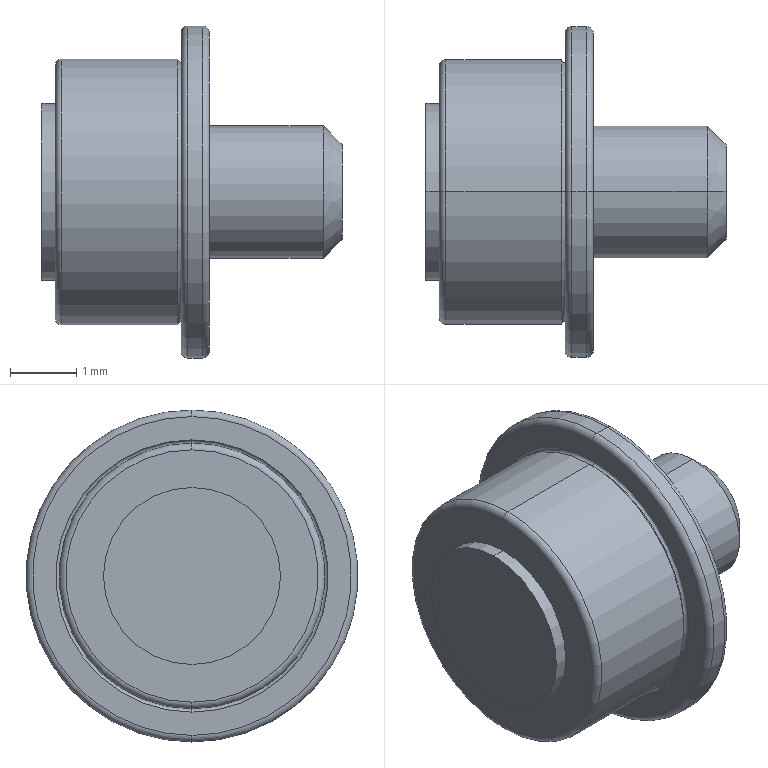Part | STEP file | Guide wheel mechanism revised.sldasm-Part-503 | 1 solid | 32 faces | box 4.52 x 5 x 5 mm | volume 39.127 mm3 | torus 14 | cylinder 10 | plane 6 | cone 2 | commonest cylinder face diameters 2 x4 2.667 x2 4 x2 5 x2
STEP:
#1=CARTESIAN_POINT('',(1.846,0.,2.));
#2=VERTEX_POINT('',#1);
#3=CARTESIAN_POINT('',(1.896,0.,1.95));
#4=VERTEX_POINT('',#3);
#5=CARTESIAN_POINT('',(1.896,0.,2.));
#6=DIRECTION('',(0.,-1.,0.));
#7=DIRECTION('',(0.,0.,-1.));
#8=AXIS2_PLACEMENT_3D('',#5,#6,#7);
#9=CIRCLE('',#8,0.05);
#10=EDGE_CURVE('',#2,#4,#9,.T.);
#11=ORIENTED_EDGE('',*,*,#10,.T.);
#12=CARTESIAN_POINT('',(1.896,0.,-1.95));
#13=VERTEX_POINT('',#12);
#14=CARTESIAN_POINT('',(1.896,0.,0.));
#15=DIRECTION('',(-1.,0.,0.));
#16=DIRECTION('',(0.,0.,1.));
#17=AXIS2_PLACEMENT_3D('',#14,#15,#16);
#18=CIRCLE('',#17,1.95);
#19=EDGE_CURVE('',#4,#13,#18,.T.);
#20=ORIENTED_EDGE('',*,*,#19,.T.);
#21=CARTESIAN_POINT('',(1.846,0.,-2.));
#22=VERTEX_POINT('',#21);
#23=CARTESIAN_POINT('',(1.896,0.,-2.));
#24=DIRECTION('',(0.,1.,0.));
#25=DIRECTION('',(0.,0.,1.));
#26=AXIS2_PLACEMENT_3D('',#23,#24,#25);
#27=CIRCLE('',#26,0.05);
#28=EDGE_CURVE('',#22,#13,#27,.T.);
#29=ORIENTED_EDGE('',*,*,#28,.F.);
#30=CARTESIAN_POINT('',(1.846,0.,0.));
#31=DIRECTION('',(-1.,0.,0.));
#32=DIRECTION('',(0.,0.,1.));
#33=AXIS2_PLACEMENT_3D('',#30,#31,#32);
#34=CIRCLE('',#33,2.);
#35=EDGE_CURVE('',#2,#22,#34,.T.);
#36=ORIENTED_EDGE('',*,*,#35,.F.);
#37=EDGE_LOOP('',(#11,#20,#29,#36));
#38=FACE_OUTER_BOUND('',#37,.T.);
#39=CARTESIAN_POINT('',(1.896,0.,0.));
#40=DIRECTION('',(-1.,0.,0.));
#41=DIRECTION('',(0.,0.,1.));
#42=AXIS2_PLACEMENT_3D('',#39,#40,#41);
#43=TOROIDAL_SURFACE('',#42,2.,0.05);
#44=ADVANCED_FACE('',(#38),#43,.F.);
#45=ORIENTED_EDGE('',*,*,#28,.T.);
#46=CARTESIAN_POINT('',(1.896,0.,0.));
#47=DIRECTION('',(-1.,0.,0.));
#48=DIRECTION('',(0.,0.,1.));
#49=AXIS2_PLACEMENT_3D('',#46,#47,#48);
#50=CIRCLE('',#49,1.95);
#51=EDGE_CURVE('',#13,#4,#50,.T.);
#52=ORIENTED_EDGE('',*,*,#51,.T.);
#53=ORIENTED_EDGE('',*,*,#10,.F.);
#54=CARTESIAN_POINT('',(1.846,0.,0.));
#55=DIRECTION('',(-1.,0.,0.));
#56=DIRECTION('',(0.,0.,1.));
#57=AXIS2_PLACEMENT_3D('',#54,#55,#56);
#58=CIRCLE('',#57,2.);
#59=EDGE_CURVE('',#22,#2,#58,.T.);
#60=ORIENTED_EDGE('',*,*,#59,.F.);
#61=EDGE_LOOP('',(#45,#52,#53,#60));
#62=FACE_OUTER_BOUND('',#61,.T.);
#63=CARTESIAN_POINT('',(1.896,0.,0.));
#64=DIRECTION('',(-1.,0.,0.));
#65=DIRECTION('',(0.,0.,1.));
#66=AXIS2_PLACEMENT_3D('',#63,#64,#65);
#67=TOROIDAL_SURFACE('',#66,2.,0.05);
#68=ADVANCED_FACE('',(#62),#67,.F.);
#69=CARTESIAN_POINT('',(-0.2,0.,-1.333));
#70=VERTEX_POINT('',#69);
#71=CARTESIAN_POINT('',(-0.2,0.,1.333));
#72=VERTEX_POINT('',#71);
#73=CARTESIAN_POINT('',(-0.2,0.,0.));
#74=DIRECTION('',(1.,0.,0.));
#75=DIRECTION('',(0.,0.,-1.));
#76=AXIS2_PLACEMENT_3D('',#73,#74,#75);
#77=CIRCLE('',#76,1.333);
#78=EDGE_CURVE('',#70,#72,#77,.T.);
#79=ORIENTED_EDGE('',*,*,#78,.T.);
#80=CARTESIAN_POINT('',(0.,0.,1.333));
#81=VERTEX_POINT('',#80);
#82=CARTESIAN_POINT('',(-0.2,0.,1.333));
#83=DIRECTION('',(1.,0.,0.));
#84=VECTOR('',#83,1000.);
#85=LINE('',#82,#84);
#86=EDGE_CURVE('',#72,#81,#85,.T.);
#87=ORIENTED_EDGE('',*,*,#86,.T.);
#88=CARTESIAN_POINT('',(0.,0.,-1.333));
#89=VERTEX_POINT('',#88);
#90=CARTESIAN_POINT('',(0.,0.,0.));
#91=DIRECTION('',(-1.,0.,0.));
#92=DIRECTION('',(0.,0.,-1.));
#93=AXIS2_PLACEMENT_3D('',#90,#91,#92);
#94=CIRCLE('',#93,1.333);
#95=EDGE_CURVE('',#81,#89,#94,.T.);
#96=ORIENTED_EDGE('',*,*,#95,.T.);
#97=CARTESIAN_POINT('',(-0.2,0.,-1.333));
#98=DIRECTION('',(1.,0.,0.));
#99=VECTOR('',#98,1000.);
#100=LINE('',#97,#99);
#101=EDGE_CURVE('',#70,#89,#100,.T.);
#102=ORIENTED_EDGE('',*,*,#101,.F.);
#103=EDGE_LOOP('',(#79,#87,#96,#102));
#104=FACE_OUTER_BOUND('',#103,.T.);
#105=CARTESIAN_POINT('',(-0.2,0.,0.));
#106=DIRECTION('',(1.,0.,0.));
#107=DIRECTION('',(0.,0.,-1.));
#108=AXIS2_PLACEMENT_3D('',#105,#106,#107);
#109=CYLINDRICAL_SURFACE('',#108,1.333);
#110=ADVANCED_FACE('',(#104),#109,.T.);
#111=CARTESIAN_POINT('',(4.32,0.,-0.7151));
#112=VERTEX_POINT('',#111);
#113=CARTESIAN_POINT('',(4.32,0.,0.7151));
#114=VERTEX_POINT('',#113);
#115=CARTESIAN_POINT('',(4.32,0.,0.));
#116=DIRECTION('',(1.,0.,0.));
#117=DIRECTION('',(0.,0.,-1.));
#118=AXIS2_PLACEMENT_3D('',#115,#116,#117);
#119=CIRCLE('',#118,0.7151);
#120=EDGE_CURVE('',#112,#114,#119,.T.);
#121=ORIENTED_EDGE('',*,*,#120,.F.);
#122=CARTESIAN_POINT('',(4.035,0.,-1.));
#123=VERTEX_POINT('',#122);
#124=CARTESIAN_POINT('',(4.035,0.,-1.));
#125=DIRECTION('',(-0.7071,0.,-0.7071));
#126=VECTOR('',#125,1000.);
#127=LINE('',#124,#126);
#128=EDGE_CURVE('',#112,#123,#127,.T.);
#129=ORIENTED_EDGE('',*,*,#128,.T.);
#130=CARTESIAN_POINT('',(4.035,0.,1.));
#131=VERTEX_POINT('',#130);
#132=CARTESIAN_POINT('',(4.035,0.,0.));
#133=DIRECTION('',(1.,0.,0.));
#134=DIRECTION('',(0.,0.,-1.));
#135=AXIS2_PLACEMENT_3D('',#132,#133,#134);
#136=CIRCLE('',#135,1.);
#137=EDGE_CURVE('',#123,#131,#136,.T.);
#138=ORIENTED_EDGE('',*,*,#137,.T.);
#139=CARTESIAN_POINT('',(4.035,0.,1.));
#140=DIRECTION('',(-0.7071,0.,0.7071));
#141=VECTOR('',#140,1000.);
#142=LINE('',#139,#141);
#143=EDGE_CURVE('',#114,#131,#142,.T.);
#144=ORIENTED_EDGE('',*,*,#143,.F.);
#145=EDGE_LOOP('',(#121,#129,#138,#144));
#146=FACE_OUTER_BOUND('',#145,.T.);
#147=CARTESIAN_POINT('',(4.035,0.,0.));
#148=DIRECTION('',(-1.,0.,0.));
#149=DIRECTION('',(0.,0.,1.));
#150=AXIS2_PLACEMENT_3D('',#147,#148,#149);
#151=CONICAL_SURFACE('',#150,1.,0.7854);
#152=ADVANCED_FACE('',(#146),#151,.T.);
#153=CARTESIAN_POINT('',(2.22,0.,1.));
#154=VERTEX_POINT('',#153);
#155=CARTESIAN_POINT('',(2.22,0.,-1.));
#156=VERTEX_POINT('',#155);
#157=CARTESIAN_POINT('',(2.22,0.,0.));
#158=DIRECTION('',(-1.,0.,0.));
#159=DIRECTION('',(0.,0.,-1.));
#160=AXIS2_PLACEMENT_3D('',#157,#158,#159);
#161=CIRCLE('',#160,1.);
#162=EDGE_CURVE('',#154,#156,#161,.T.);
#163=ORIENTED_EDGE('',*,*,#162,.F.);
#164=CARTESIAN_POINT('',(-0.2,0.,1.));
#165=DIRECTION('',(1.,0.,0.));
#166=VECTOR('',#165,1000.);
#167=LINE('',#164,#166);
#168=EDGE_CURVE('',#154,#131,#167,.T.);
#169=ORIENTED_EDGE('',*,*,#168,.T.);
#170=ORIENTED_EDGE('',*,*,#137,.F.);
#171=CARTESIAN_POINT('',(-0.2,0.,-1.));
#172=DIRECTION('',(1.,0.,0.));
#173=VECTOR('',#172,1000.);
#174=LINE('',#171,#173);
#175=EDGE_CURVE('',#156,#123,#174,.T.);
#176=ORIENTED_EDGE('',*,*,#175,.F.);
#177=EDGE_LOOP('',(#163,#169,#170,#176));
#178=FACE_OUTER_BOUND('',#177,.T.);
#179=CARTESIAN_POINT('',(-0.2,0.,0.));
#180=DIRECTION('',(1.,0.,0.));
#181=DIRECTION('',(0.,0.,-1.));
#182=AXIS2_PLACEMENT_3D('',#179,#180,#181);
#183=CYLINDRICAL_SURFACE('',#182,1.);
#184=ADVANCED_FACE('',(#178),#183,.T.);
#185=ORIENTED_EDGE('',*,*,#35,.T.);
#186=CARTESIAN_POINT('',(0.1,0.,-2.));
#187=VERTEX_POINT('',#186);
#188=CARTESIAN_POINT('',(2.32,0.,-2.));
#189=DIRECTION('',(-1.,0.,0.));
#190=VECTOR('',#189,1000.);
#191=LINE('',#188,#190);
#192=EDGE_CURVE('',#22,#187,#191,.T.);
#193=ORIENTED_EDGE('',*,*,#192,.T.);
#194=CARTESIAN_POINT('',(0.1,0.,2.));
#195=VERTEX_POINT('',#194);
#196=CARTESIAN_POINT('',(0.1,0.,0.));
#197=DIRECTION('',(-1.,0.,0.));
#198=DIRECTION('',(0.,0.,1.));
#199=AXIS2_PLACEMENT_3D('',#196,#197,#198);
#200=CIRCLE('',#199,2.);
#201=EDGE_CURVE('',#195,#187,#200,.T.);
#202=ORIENTED_EDGE('',*,*,#201,.F.);
#203=CARTESIAN_POINT('',(2.32,0.,2.));
#204=DIRECTION('',(-1.,0.,0.));
#205=VECTOR('',#204,1000.);
#206=LINE('',#203,#205);
#207=EDGE_CURVE('',#2,#195,#206,.T.);
#208=ORIENTED_EDGE('',*,*,#207,.F.);
#209=EDGE_LOOP('',(#185,#193,#202,#208));
#210=FACE_OUTER_BOUND('',#209,.T.);
#211=CARTESIAN_POINT('',(2.32,0.,0.));
#212=DIRECTION('',(-1.,0.,0.));
#213=DIRECTION('',(0.,0.,1.));
#214=AXIS2_PLACEMENT_3D('',#211,#212,#213);
#215=CYLINDRICAL_SURFACE('',#214,2.);
#216=ADVANCED_FACE('',(#210),#215,.T.);
#217=ORIENTED_EDGE('',*,*,#51,.F.);
#218=CARTESIAN_POINT('',(1.896,0.,-2.05));
#219=VERTEX_POINT('',#218);
#220=CARTESIAN_POINT('',(1.896,0.,-2.));
#221=DIRECTION('',(0.,1.,0.));
#222=DIRECTION('',(0.,0.,1.));
#223=AXIS2_PLACEMENT_3D('',#220,#221,#222);
#224=CIRCLE('',#223,0.05);
#225=EDGE_CURVE('',#13,#219,#224,.T.);
#226=ORIENTED_EDGE('',*,*,#225,.T.);
#227=CARTESIAN_POINT('',(1.896,0.,2.05));
#228=VERTEX_POINT('',#227);
#229=CARTESIAN_POINT('',(1.896,0.,0.));
#230=DIRECTION('',(-1.,0.,0.));
#231=DIRECTION('',(0.,0.,1.));
#232=AXIS2_PLACEMENT_3D('',#229,#230,#231);
#233=CIRCLE('',#232,2.05);
#234=EDGE_CURVE('',#219,#228,#233,.T.);
#235=ORIENTED_EDGE('',*,*,#234,.T.);
#236=CARTESIAN_POINT('',(1.896,0.,2.));
#237=DIRECTION('',(0.,-1.,0.));
#238=DIRECTION('',(0.,0.,-1.));
#239=AXIS2_PLACEMENT_3D('',#236,#237,#238);
#240=CIRCLE('',#239,0.05);
#241=EDGE_CURVE('',#4,#228,#240,.T.);
#242=ORIENTED_EDGE('',*,*,#241,.F.);
#243=EDGE_LOOP('',(#217,#226,#235,#242));
#244=FACE_OUTER_BOUND('',#243,.T.);
#245=CARTESIAN_POINT('',(1.896,0.,0.));
#246=DIRECTION('',(-1.,0.,0.));
#247=DIRECTION('',(0.,0.,1.));
#248=AXIS2_PLACEMENT_3D('',#245,#246,#247);
#249=TOROIDAL_SURFACE('',#248,2.,0.05);
#250=ADVANCED_FACE('',(#244),#249,.F.);
#251=CARTESIAN_POINT('',(1.996,0.,2.5));
#252=VERTEX_POINT('',#251);
#253=CARTESIAN_POINT('',(1.996,0.,-2.5));
#254=VERTEX_POINT('',#253);
#255=CARTESIAN_POINT('',(1.996,0.,0.));
#256=DIRECTION('',(-1.,0.,0.));
#257=DIRECTION('',(0.,0.,1.));
#258=AXIS2_PLACEMENT_3D('',#255,#256,#257);
#259=CIRCLE('',#258,2.5);
#260=EDGE_CURVE('',#252,#254,#259,.T.);
#261=ORIENTED_EDGE('',*,*,#260,.T.);
#262=CARTESIAN_POINT('',(1.896,0.,-2.4));
#263=VERTEX_POINT('',#262);
#264=CARTESIAN_POINT('',(1.996,0.,-2.4));
#265=DIRECTION('',(0.,1.,0.));
#266=DIRECTION('',(0.,0.,1.));
#267=AXIS2_PLACEMENT_3D('',#264,#265,#266);
#268=CIRCLE('',#267,0.1);
#269=EDGE_CURVE('',#254,#263,#268,.T.);
#270=ORIENTED_EDGE('',*,*,#269,.T.);
#271=CARTESIAN_POINT('',(1.896,0.,2.4));
#272=VERTEX_POINT('',#271);
#273=CARTESIAN_POINT('',(1.896,0.,0.));
#274=DIRECTION('',(-1.,0.,0.));
#275=DIRECTION('',(0.,0.,1.));
#276=AXIS2_PLACEMENT_3D('',#273,#274,#275);
#277=CIRCLE('',#276,2.4);
#278=EDGE_CURVE('',#272,#263,#277,.T.);
#279=ORIENTED_EDGE('',*,*,#278,.F.);
#280=CARTESIAN_POINT('',(1.996,0.,2.4));
#281=DIRECTION('',(0.,-1.,0.));
#282=DIRECTION('',(0.,0.,-1.));
#283=AXIS2_PLACEMENT_3D('',#280,#281,#282);
#284=CIRCLE('',#283,0.1);
#285=EDGE_CURVE('',#252,#272,#284,.T.);
#286=ORIENTED_EDGE('',*,*,#285,.F.);
#287=EDGE_LOOP('',(#261,#270,#279,#286));
#288=FACE_OUTER_BOUND('',#287,.T.);
#289=CARTESIAN_POINT('',(1.996,0.,0.));
#290=DIRECTION('',(-1.,0.,0.));
#291=DIRECTION('',(0.,0.,1.));
#292=AXIS2_PLACEMENT_3D('',#289,#290,#291);
#293=TOROIDAL_SURFACE('',#292,2.4,0.1);
#294=ADVANCED_FACE('',(#288),#293,.T.);
#295=CARTESIAN_POINT('',(2.22,0.,2.5));
#296=VERTEX_POINT('',#295);
#297=CARTESIAN_POINT('',(2.22,0.,-2.5));
#298=VERTEX_POINT('',#297);
#299=CARTESIAN_POINT('',(2.22,0.,0.));
#300=DIRECTION('',(-1.,0.,0.));
#301=DIRECTION('',(0.,0.,1.));
#302=AXIS2_PLACEMENT_3D('',#299,#300,#301);
#303=CIRCLE('',#302,2.5);
#304=EDGE_CURVE('',#296,#298,#303,.T.);
#305=ORIENTED_EDGE('',*,*,#304,.T.);
#306=CARTESIAN_POINT('',(2.32,0.,-2.5));
#307=DIRECTION('',(-1.,0.,0.));
#308=VECTOR('',#307,1000.);
#309=LINE('',#306,#308);
#310=EDGE_CURVE('',#298,#254,#309,.T.);
#311=ORIENTED_EDGE('',*,*,#310,.T.);
#312=ORIENTED_EDGE('',*,*,#260,.F.);
#313=CARTESIAN_POINT('',(2.32,0.,2.5));
#314=DIRECTION('',(-1.,0.,0.));
#315=VECTOR('',#314,1000.);
#316=LINE('',#313,#315);
#317=EDGE_CURVE('',#296,#252,#316,.T.);
#318=ORIENTED_EDGE('',*,*,#317,.F.);
#319=EDGE_LOOP('',(#305,#311,#312,#318));
#320=FACE_OUTER_BOUND('',#319,.T.);
#321=CARTESIAN_POINT('',(2.32,0.,0.));
#322=DIRECTION('',(-1.,0.,0.));
#323=DIRECTION('',(0.,0.,1.));
#324=AXIS2_PLACEMENT_3D('',#321,#322,#323);
#325=CYLINDRICAL_SURFACE('',#324,2.5);
#326=ADVANCED_FACE('',(#320),#325,.T.);
#327=CARTESIAN_POINT('',(2.32,0.,2.4));
#328=VERTEX_POINT('',#327);
#329=CARTESIAN_POINT('',(2.32,0.,-2.4));
#330=VERTEX_POINT('',#329);
#331=CARTESIAN_POINT('',(2.32,0.,0.));
#332=DIRECTION('',(-1.,0.,0.));
#333=DIRECTION('',(0.,0.,1.));
#334=AXIS2_PLACEMENT_3D('',#331,#332,#333);
#335=CIRCLE('',#334,2.4);
#336=EDGE_CURVE('',#328,#330,#335,.T.);
#337=ORIENTED_EDGE('',*,*,#336,.T.);
#338=CARTESIAN_POINT('',(2.22,0.,-2.4));
#339=DIRECTION('',(0.,1.,0.));
#340=DIRECTION('',(0.,0.,1.));
#341=AXIS2_PLACEMENT_3D('',#338,#339,#340);
#342=CIRCLE('',#341,0.1);
#343=EDGE_CURVE('',#330,#298,#342,.T.);
#344=ORIENTED_EDGE('',*,*,#343,.T.);
#345=ORIENTED_EDGE('',*,*,#304,.F.);
#346=CARTESIAN_POINT('',(2.22,0.,2.4));
#347=DIRECTION('',(0.,-1.,0.));
#348=DIRECTION('',(0.,0.,-1.));
#349=AXIS2_PLACEMENT_3D('',#346,#347,#348);
#350=CIRCLE('',#349,0.1);
#351=EDGE_CURVE('',#328,#296,#350,.T.);
#352=ORIENTED_EDGE('',*,*,#351,.F.);
#353=EDGE_LOOP('',(#337,#344,#345,#352));
#354=FACE_OUTER_BOUND('',#353,.T.);
#355=CARTESIAN_POINT('',(2.22,0.,0.));
#356=DIRECTION('',(-1.,0.,0.));
#357=DIRECTION('',(0.,0.,1.));
#358=AXIS2_PLACEMENT_3D('',#355,#356,#357);
#359=TOROIDAL_SURFACE('',#358,2.4,0.1);
#360=ADVANCED_FACE('',(#354),#359,.T.);
#361=ORIENTED_EDGE('',*,*,#162,.T.);
#362=CARTESIAN_POINT('',(2.32,0.,-1.1));
#363=VERTEX_POINT('',#362);
#364=CARTESIAN_POINT('',(2.22,0.,-1.1));
#365=DIRECTION('',(0.,1.,0.));
#366=DIRECTION('',(0.,0.,1.));
#367=AXIS2_PLACEMENT_3D('',#364,#365,#366);
#368=CIRCLE('',#367,0.1);
#369=EDGE_CURVE('',#156,#363,#368,.T.);
#370=ORIENTED_EDGE('',*,*,#369,.T.);
#371=CARTESIAN_POINT('',(2.32,0.,1.1));
#372=VERTEX_POINT('',#371);
#373=CARTESIAN_POINT('',(2.32,0.,0.));
#374=DIRECTION('',(-1.,0.,0.));
#375=DIRECTION('',(0.,0.,1.));
#376=AXIS2_PLACEMENT_3D('',#373,#374,#375);
#377=CIRCLE('',#376,1.1);
#378=EDGE_CURVE('',#372,#363,#377,.T.);
#379=ORIENTED_EDGE('',*,*,#378,.F.);
#380=CARTESIAN_POINT('',(2.22,0.,1.1));
#381=DIRECTION('',(0.,-1.,0.));
#382=DIRECTION('',(0.,0.,-1.));
#383=AXIS2_PLACEMENT_3D('',#380,#381,#382);
#384=CIRCLE('',#383,0.1);
#385=EDGE_CURVE('',#154,#372,#384,.T.);
#386=ORIENTED_EDGE('',*,*,#385,.F.);
#387=EDGE_LOOP('',(#361,#370,#379,#386));
#388=FACE_OUTER_BOUND('',#387,.T.);
#389=CARTESIAN_POINT('',(2.22,0.,0.));
#390=DIRECTION('',(-1.,0.,0.));
#391=DIRECTION('',(0.,0.,1.));
#392=AXIS2_PLACEMENT_3D('',#389,#390,#391);
#393=TOROIDAL_SURFACE('',#392,1.1,0.1);
#394=ADVANCED_FACE('',(#388),#393,.T.);
#395=ORIENTED_EDGE('',*,*,#201,.T.);
#396=CARTESIAN_POINT('',(0.,0.,-1.9));
#397=VERTEX_POINT('',#396);
#398=CARTESIAN_POINT('',(0.1,0.,-1.9));
#399=DIRECTION('',(0.,1.,0.));
#400=DIRECTION('',(0.,0.,1.));
#401=AXIS2_PLACEMENT_3D('',#398,#399,#400);
#402=CIRCLE('',#401,0.1);
#403=EDGE_CURVE('',#187,#397,#402,.T.);
#404=ORIENTED_EDGE('',*,*,#403,.T.);
#405=CARTESIAN_POINT('',(0.,0.,1.9));
#406=VERTEX_POINT('',#405);
#407=CARTESIAN_POINT('',(0.,0.,0.));
#408=DIRECTION('',(-1.,0.,0.));
#409=DIRECTION('',(0.,0.,1.));
#410=AXIS2_PLACEMENT_3D('',#407,#408,#409);
#411=CIRCLE('',#410,1.9);
#412=EDGE_CURVE('',#406,#397,#411,.T.);
#413=ORIENTED_EDGE('',*,*,#412,.F.);
#414=CARTESIAN_POINT('',(0.1,0.,1.9));
#415=DIRECTION('',(0.,-1.,0.));
#416=DIRECTION('',(0.,0.,-1.));
#417=AXIS2_PLACEMENT_3D('',#414,#415,#416);
#418=CIRCLE('',#417,0.1);
#419=EDGE_CURVE('',#195,#406,#418,.T.);
#420=ORIENTED_EDGE('',*,*,#419,.F.);
#421=EDGE_LOOP('',(#395,#404,#413,#420));
#422=FACE_OUTER_BOUND('',#421,.T.);
#423=CARTESIAN_POINT('',(0.1,0.,0.));
#424=DIRECTION('',(-1.,0.,0.));
#425=DIRECTION('',(0.,0.,1.));
#426=AXIS2_PLACEMENT_3D('',#423,#424,#425);
#427=TOROIDAL_SURFACE('',#426,1.9,0.1);
#428=ADVANCED_FACE('',(#422),#427,.T.);
#429=ORIENTED_EDGE('',*,*,#412,.T.);
#430=CARTESIAN_POINT('',(0.,0.,0.));
#431=DIRECTION('',(-1.,0.,0.));
#432=DIRECTION('',(0.,0.,1.));
#433=AXIS2_PLACEMENT_3D('',#430,#431,#432);
#434=CIRCLE('',#433,1.9);
#435=EDGE_CURVE('',#397,#406,#434,.T.);
#436=ORIENTED_EDGE('',*,*,#435,.T.);
#437=EDGE_LOOP('',(#429,#436));
#438=FACE_OUTER_BOUND('',#437,.T.);
#439=CARTESIAN_POINT('',(0.,0.,0.));
#440=DIRECTION('',(-1.,0.,0.));
#441=DIRECTION('',(0.,0.,-1.));
#442=AXIS2_PLACEMENT_3D('',#439,#440,#441);
#443=CIRCLE('',#442,1.333);
#444=EDGE_CURVE('',#89,#81,#443,.T.);
#445=ORIENTED_EDGE('',*,*,#444,.F.);
#446=ORIENTED_EDGE('',*,*,#95,.F.);
#447=EDGE_LOOP('',(#445,#446));
#448=FACE_BOUND('',#447,.T.);
#449=CARTESIAN_POINT('',(0.,1.9,0.));
#450=DIRECTION('',(1.,0.,0.));
#451=DIRECTION('',(0.,0.,-1.));
#452=AXIS2_PLACEMENT_3D('',#449,#450,#451);
#453=PLANE('',#452);
#454=ADVANCED_FACE('',(#438,#448),#453,.F.);
#455=ORIENTED_EDGE('',*,*,#403,.F.);
#456=CARTESIAN_POINT('',(0.1,0.,0.));
#457=DIRECTION('',(-1.,0.,0.));
#458=DIRECTION('',(0.,0.,1.));
#459=AXIS2_PLACEMENT_3D('',#456,#457,#458);
#460=CIRCLE('',#459,2.);
#461=EDGE_CURVE('',#187,#195,#460,.T.);
#462=ORIENTED_EDGE('',*,*,#461,.T.);
#463=ORIENTED_EDGE('',*,*,#419,.T.);
#464=ORIENTED_EDGE('',*,*,#435,.F.);
#465=EDGE_LOOP('',(#455,#462,#463,#464));
#466=FACE_OUTER_BOUND('',#465,.T.);
#467=CARTESIAN_POINT('',(0.1,0.,0.));
#468=DIRECTION('',(-1.,0.,0.));
#469=DIRECTION('',(0.,0.,1.));
#470=AXIS2_PLACEMENT_3D('',#467,#468,#469);
#471=TOROIDAL_SURFACE('',#470,1.9,0.1);
#472=ADVANCED_FACE('',(#466),#471,.T.);
#473=ORIENTED_EDGE('',*,*,#369,.F.);
#474=CARTESIAN_POINT('',(2.22,0.,0.));
#475=DIRECTION('',(-1.,0.,0.));
#476=DIRECTION('',(0.,0.,-1.));
#477=AXIS2_PLACEMENT_3D('',#474,#475,#476);
#478=CIRCLE('',#477,1.);
#479=EDGE_CURVE('',#156,#154,#478,.T.);
#480=ORIENTED_EDGE('',*,*,#479,.T.);
#481=ORIENTED_EDGE('',*,*,#385,.T.);
#482=CARTESIAN_POINT('',(2.32,0.,0.));
#483=DIRECTION('',(-1.,0.,0.));
#484=DIRECTION('',(0.,0.,1.));
#485=AXIS2_PLACEMENT_3D('',#482,#483,#484);
#486=CIRCLE('',#485,1.1);
#487=EDGE_CURVE('',#363,#372,#486,.T.);
#488=ORIENTED_EDGE('',*,*,#487,.F.);
#489=EDGE_LOOP('',(#473,#480,#481,#488));
#490=FACE_OUTER_BOUND('',#489,.T.);
#491=CARTESIAN_POINT('',(2.22,0.,0.));
#492=DIRECTION('',(-1.,0.,0.));
#493=DIRECTION('',(0.,0.,1.));
#494=AXIS2_PLACEMENT_3D('',#491,#492,#493);
#495=TOROIDAL_SURFACE('',#494,1.1,0.1);
#496=ADVANCED_FACE('',(#490),#495,.T.);
#497=ORIENTED_EDGE('',*,*,#336,.F.);
#498=CARTESIAN_POINT('',(2.32,0.,0.));
#499=DIRECTION('',(-1.,0.,0.));
#500=DIRECTION('',(0.,0.,1.));
#501=AXIS2_PLACEMENT_3D('',#498,#499,#500);
#502=CIRCLE('',#501,2.4);
#503=EDGE_CURVE('',#330,#328,#502,.T.);
#504=ORIENTED_EDGE('',*,*,#503,.F.);
#505=EDGE_LOOP('',(#497,#504));
#506=FACE_OUTER_BOUND('',#505,.T.);
#507=ORIENTED_EDGE('',*,*,#378,.T.);
#508=ORIENTED_EDGE('',*,*,#487,.T.);
#509=EDGE_LOOP('',(#507,#508));
#510=FACE_BOUND('',#509,.T.);
#511=CARTESIAN_POINT('',(2.32,1.1,0.));
#512=DIRECTION('',(-1.,0.,0.));
#513=DIRECTION('',(0.,0.,1.));
#514=AXIS2_PLACEMENT_3D('',#511,#512,#513);
#515=PLANE('',#514);
#516=ADVANCED_FACE('',(#506,#510),#515,.F.);
#517=ORIENTED_EDGE('',*,*,#343,.F.);
#518=ORIENTED_EDGE('',*,*,#503,.T.);
#519=ORIENTED_EDGE('',*,*,#351,.T.);
#520=CARTESIAN_POINT('',(2.22,0.,0.));
#521=DIRECTION('',(-1.,0.,0.));
#522=DIRECTION('',(0.,0.,1.));
#523=AXIS2_PLACEMENT_3D('',#520,#521,#522);
#524=CIRCLE('',#523,2.5);
#525=EDGE_CURVE('',#298,#296,#524,.T.);
#526=ORIENTED_EDGE('',*,*,#525,.F.);
#527=EDGE_LOOP('',(#517,#518,#519,#526));
#528=FACE_OUTER_BOUND('',#527,.T.);
#529=CARTESIAN_POINT('',(2.22,0.,0.));
#530=DIRECTION('',(-1.,0.,0.));
#531=DIRECTION('',(0.,0.,1.));
#532=AXIS2_PLACEMENT_3D('',#529,#530,#531);
#533=TOROIDAL_SURFACE('',#532,2.4,0.1);
#534=ADVANCED_FACE('',(#528),#533,.T.);
#535=ORIENTED_EDGE('',*,*,#310,.F.);
#536=ORIENTED_EDGE('',*,*,#525,.T.);
#537=ORIENTED_EDGE('',*,*,#317,.T.);
#538=CARTESIAN_POINT('',(1.996,0.,0.));
#539=DIRECTION('',(-1.,0.,0.));
#540=DIRECTION('',(0.,0.,1.));
#541=AXIS2_PLACEMENT_3D('',#538,#539,#540);
#542=CIRCLE('',#541,2.5);
#543=EDGE_CURVE('',#254,#252,#542,.T.);
#544=ORIENTED_EDGE('',*,*,#543,.F.);
#545=EDGE_LOOP('',(#535,#536,#537,#544));
#546=FACE_OUTER_BOUND('',#545,.T.);
#547=CARTESIAN_POINT('',(2.32,0.,0.));
#548=DIRECTION('',(-1.,0.,0.));
#549=DIRECTION('',(0.,0.,1.));
#550=AXIS2_PLACEMENT_3D('',#547,#548,#549);
#551=CYLINDRICAL_SURFACE('',#550,2.5);
#552=ADVANCED_FACE('',(#546),#551,.T.);
#553=ORIENTED_EDGE('',*,*,#269,.F.);
#554=ORIENTED_EDGE('',*,*,#543,.T.);
#555=ORIENTED_EDGE('',*,*,#285,.T.);
#556=CARTESIAN_POINT('',(1.896,0.,0.));
#557=DIRECTION('',(-1.,0.,0.));
#558=DIRECTION('',(0.,0.,1.));
#559=AXIS2_PLACEMENT_3D('',#556,#557,#558);
#560=CIRCLE('',#559,2.4);
#561=EDGE_CURVE('',#263,#272,#560,.T.);
#562=ORIENTED_EDGE('',*,*,#561,.F.);
#563=EDGE_LOOP('',(#553,#554,#555,#562));
#564=FACE_OUTER_BOUND('',#563,.T.);
#565=CARTESIAN_POINT('',(1.996,0.,0.));
#566=DIRECTION('',(-1.,0.,0.));
#567=DIRECTION('',(0.,0.,1.));
#568=AXIS2_PLACEMENT_3D('',#565,#566,#567);
#569=TOROIDAL_SURFACE('',#568,2.4,0.1);
#570=ADVANCED_FACE('',(#564),#569,.T.);
#571=CARTESIAN_POINT('',(1.896,0.,0.));
#572=DIRECTION('',(-1.,0.,0.));
#573=DIRECTION('',(0.,0.,1.));
#574=AXIS2_PLACEMENT_3D('',#571,#572,#573);
#575=CIRCLE('',#574,2.05);
#576=EDGE_CURVE('',#228,#219,#575,.T.);
#577=ORIENTED_EDGE('',*,*,#576,.F.);
#578=ORIENTED_EDGE('',*,*,#234,.F.);
#579=EDGE_LOOP('',(#577,#578));
#580=FACE_BOUND('',#579,.T.);
#581=ORIENTED_EDGE('',*,*,#278,.T.);
#582=ORIENTED_EDGE('',*,*,#561,.T.);
#583=EDGE_LOOP('',(#581,#582));
#584=FACE_OUTER_BOUND('',#583,.T.);
#585=CARTESIAN_POINT('',(1.896,2.4,0.));
#586=DIRECTION('',(1.,0.,0.));
#587=DIRECTION('',(0.,0.,-1.));
#588=AXIS2_PLACEMENT_3D('',#585,#586,#587);
#589=PLANE('',#588);
#590=ADVANCED_FACE('',(#580,#584),#589,.F.);
#591=ORIENTED_EDGE('',*,*,#19,.F.);
#592=ORIENTED_EDGE('',*,*,#241,.T.);
#593=ORIENTED_EDGE('',*,*,#576,.T.);
#594=ORIENTED_EDGE('',*,*,#225,.F.);
#595=EDGE_LOOP('',(#591,#592,#593,#594));
#596=FACE_OUTER_BOUND('',#595,.T.);
#597=CARTESIAN_POINT('',(1.896,0.,0.));
#598=DIRECTION('',(-1.,0.,0.));
#599=DIRECTION('',(0.,0.,1.));
#600=AXIS2_PLACEMENT_3D('',#597,#598,#599);
#601=TOROIDAL_SURFACE('',#600,2.,0.05);
#602=ADVANCED_FACE('',(#596),#601,.F.);
#603=ORIENTED_EDGE('',*,*,#192,.F.);
#604=ORIENTED_EDGE('',*,*,#59,.T.);
#605=ORIENTED_EDGE('',*,*,#207,.T.);
#606=ORIENTED_EDGE('',*,*,#461,.F.);
#607=EDGE_LOOP('',(#603,#604,#605,#606));
#608=FACE_OUTER_BOUND('',#607,.T.);
#609=CARTESIAN_POINT('',(2.32,0.,0.));
#610=DIRECTION('',(-1.,0.,0.));
#611=DIRECTION('',(0.,0.,1.));
#612=AXIS2_PLACEMENT_3D('',#609,#610,#611);
#613=CYLINDRICAL_SURFACE('',#612,2.);
#614=ADVANCED_FACE('',(#608),#613,.T.);
#615=ORIENTED_EDGE('',*,*,#168,.F.);
#616=ORIENTED_EDGE('',*,*,#479,.F.);
#617=ORIENTED_EDGE('',*,*,#175,.T.);
#618=CARTESIAN_POINT('',(4.035,0.,0.));
#619=DIRECTION('',(1.,0.,0.));
#620=DIRECTION('',(0.,0.,-1.));
#621=AXIS2_PLACEMENT_3D('',#618,#619,#620);
#622=CIRCLE('',#621,1.);
#623=EDGE_CURVE('',#131,#123,#622,.T.);
#624=ORIENTED_EDGE('',*,*,#623,.F.);
#625=EDGE_LOOP('',(#615,#616,#617,#624));
#626=FACE_OUTER_BOUND('',#625,.T.);
#627=CARTESIAN_POINT('',(-0.2,0.,0.));
#628=DIRECTION('',(1.,0.,0.));
#629=DIRECTION('',(0.,0.,-1.));
#630=AXIS2_PLACEMENT_3D('',#627,#628,#629);
#631=CYLINDRICAL_SURFACE('',#630,1.);
#632=ADVANCED_FACE('',(#626),#631,.T.);
#633=ORIENTED_EDGE('',*,*,#128,.F.);
#634=CARTESIAN_POINT('',(4.32,0.,0.));
#635=DIRECTION('',(1.,0.,0.));
#636=DIRECTION('',(0.,0.,-1.));
#637=AXIS2_PLACEMENT_3D('',#634,#635,#636);
#638=CIRCLE('',#637,0.7151);
#639=EDGE_CURVE('',#114,#112,#638,.T.);
#640=ORIENTED_EDGE('',*,*,#639,.F.);
#641=ORIENTED_EDGE('',*,*,#143,.T.);
#642=ORIENTED_EDGE('',*,*,#623,.T.);
#643=EDGE_LOOP('',(#633,#640,#641,#642));
#644=FACE_OUTER_BOUND('',#643,.T.);
#645=CARTESIAN_POINT('',(4.035,0.,0.));
#646=DIRECTION('',(-1.,0.,0.));
#647=DIRECTION('',(0.,0.,1.));
#648=AXIS2_PLACEMENT_3D('',#645,#646,#647);
#649=CONICAL_SURFACE('',#648,1.,0.7854);
#650=ADVANCED_FACE('',(#644),#649,.T.);
#651=ORIENTED_EDGE('',*,*,#639,.T.);
#652=ORIENTED_EDGE('',*,*,#120,.T.);
#653=EDGE_LOOP('',(#651,#652));
#654=FACE_OUTER_BOUND('',#653,.T.);
#655=CARTESIAN_POINT('',(4.32,0.,0.));
#656=DIRECTION('',(-1.,0.,0.));
#657=DIRECTION('',(0.,0.,1.));
#658=AXIS2_PLACEMENT_3D('',#655,#656,#657);
#659=PLANE('',#658);
#660=ADVANCED_FACE('',(#654),#659,.F.);
#661=ORIENTED_EDGE('',*,*,#86,.F.);
#662=CARTESIAN_POINT('',(-0.2,0.,0.));
#663=DIRECTION('',(1.,0.,0.));
#664=DIRECTION('',(0.,0.,-1.));
#665=AXIS2_PLACEMENT_3D('',#662,#663,#664);
#666=CIRCLE('',#665,1.333);
#667=EDGE_CURVE('',#72,#70,#666,.T.);
#668=ORIENTED_EDGE('',*,*,#667,.T.);
#669=ORIENTED_EDGE('',*,*,#101,.T.);
#670=ORIENTED_EDGE('',*,*,#444,.T.);
#671=EDGE_LOOP('',(#661,#668,#669,#670));
#672=FACE_OUTER_BOUND('',#671,.T.);
#673=CARTESIAN_POINT('',(-0.2,0.,0.));
#674=DIRECTION('',(1.,0.,0.));
#675=DIRECTION('',(0.,0.,-1.));
#676=AXIS2_PLACEMENT_3D('',#673,#674,#675);
#677=CYLINDRICAL_SURFACE('',#676,1.333);
#678=ADVANCED_FACE('',(#672),#677,.T.);
#679=ORIENTED_EDGE('',*,*,#78,.F.);
#680=ORIENTED_EDGE('',*,*,#667,.F.);
#681=EDGE_LOOP('',(#679,#680));
#682=FACE_OUTER_BOUND('',#681,.T.);
#683=CARTESIAN_POINT('',(-0.2,0.,1.333));
#684=DIRECTION('',(1.,0.,0.));
#685=DIRECTION('',(0.,0.,-1.));
#686=AXIS2_PLACEMENT_3D('',#683,#684,#685);
#687=PLANE('',#686);
#688=ADVANCED_FACE('',(#682),#687,.F.);
#689=CLOSED_SHELL('',(#44,#68,#110,#152,#184,#216,#250,#294,#326,#360,#394,#428,#454,#472,#496,#516,#534,#552,#570,#590,#602,#614,#632,#650,#660,#678,#688));
#690=CARTESIAN_POINT('',(0.,0.,-1.));
#691=VERTEX_POINT('',#690);
#692=CARTESIAN_POINT('',(0.,0.,1.));
#693=VERTEX_POINT('',#692);
#694=CARTESIAN_POINT('',(0.,0.,0.));
#695=DIRECTION('',(1.,0.,0.));
#696=DIRECTION('',(0.,0.,-1.));
#697=AXIS2_PLACEMENT_3D('',#694,#695,#696);
#698=CIRCLE('',#697,1.);
#699=EDGE_CURVE('',#691,#693,#698,.T.);
#700=ORIENTED_EDGE('',*,*,#699,.T.);
#701=CARTESIAN_POINT('',(0.1,0.,1.));
#702=VERTEX_POINT('',#701);
#703=CARTESIAN_POINT('',(-0.2,0.,1.));
#704=DIRECTION('',(1.,0.,0.));
#705=VECTOR('',#704,1000.);
#706=LINE('',#703,#705);
#707=EDGE_CURVE('',#693,#702,#706,.T.);
#708=ORIENTED_EDGE('',*,*,#707,.T.);
#709=CARTESIAN_POINT('',(0.1,0.,-1.));
#710=VERTEX_POINT('',#709);
#711=CARTESIAN_POINT('',(0.1,0.,0.));
#712=DIRECTION('',(-1.,0.,0.));
#713=DIRECTION('',(0.,0.,1.));
#714=AXIS2_PLACEMENT_3D('',#711,#712,#713);
#715=CIRCLE('',#714,1.);
#716=EDGE_CURVE('',#702,#710,#715,.T.);
#717=ORIENTED_EDGE('',*,*,#716,.T.);
#718=CARTESIAN_POINT('',(-0.2,0.,-1.));
#719=DIRECTION('',(1.,0.,0.));
#720=VECTOR('',#719,1000.);
#721=LINE('',#718,#720);
#722=EDGE_CURVE('',#691,#710,#721,.T.);
#723=ORIENTED_EDGE('',*,*,#722,.F.);
#724=EDGE_LOOP('',(#700,#708,#717,#723));
#725=FACE_OUTER_BOUND('',#724,.T.);
#726=CARTESIAN_POINT('',(-0.2,0.,0.));
#727=DIRECTION('',(1.,0.,0.));
#728=DIRECTION('',(0.,0.,-1.));
#729=AXIS2_PLACEMENT_3D('',#726,#727,#728);
#730=CYLINDRICAL_SURFACE('',#729,1.);
#731=ADVANCED_FACE('',(#725),#730,.T.);
#732=CARTESIAN_POINT('',(0.,0.,1.1));
#733=VERTEX_POINT('',#732);
#734=CARTESIAN_POINT('',(0.,0.,-1.1));
#735=VERTEX_POINT('',#734);
#736=CARTESIAN_POINT('',(0.,0.,0.));
#737=DIRECTION('',(-1.,0.,0.));
#738=DIRECTION('',(0.,0.,1.));
#739=AXIS2_PLACEMENT_3D('',#736,#737,#738);
#740=CIRCLE('',#739,1.1);
#741=EDGE_CURVE('',#733,#735,#740,.T.);
#742=ORIENTED_EDGE('',*,*,#741,.T.);
#743=CARTESIAN_POINT('',(0.1,0.,-1.1));
#744=DIRECTION('',(0.,1.,0.));
#745=DIRECTION('',(0.,0.,1.));
#746=AXIS2_PLACEMENT_3D('',#743,#744,#745);
#747=CIRCLE('',#746,0.1);
#748=EDGE_CURVE('',#735,#710,#747,.T.);
#749=ORIENTED_EDGE('',*,*,#748,.T.);
#750=ORIENTED_EDGE('',*,*,#716,.F.);
#751=CARTESIAN_POINT('',(0.1,0.,1.1));
#752=DIRECTION('',(0.,-1.,0.));
#753=DIRECTION('',(0.,0.,-1.));
#754=AXIS2_PLACEMENT_3D('',#751,#752,#753);
#755=CIRCLE('',#754,0.1);
#756=EDGE_CURVE('',#733,#702,#755,.T.);
#757=ORIENTED_EDGE('',*,*,#756,.F.);
#758=EDGE_LOOP('',(#742,#749,#750,#757));
#759=FACE_OUTER_BOUND('',#758,.T.);
#760=CARTESIAN_POINT('',(0.1,0.,0.));
#761=DIRECTION('',(-1.,0.,0.));
#762=DIRECTION('',(0.,0.,1.));
#763=AXIS2_PLACEMENT_3D('',#760,#761,#762);
#764=TOROIDAL_SURFACE('',#763,1.1,0.1);
#765=ADVANCED_FACE('',(#759),#764,.T.);
#766=ORIENTED_EDGE('',*,*,#748,.F.);
#767=CARTESIAN_POINT('',(0.,0.,0.));
#768=DIRECTION('',(-1.,0.,0.));
#769=DIRECTION('',(0.,0.,1.));
#770=AXIS2_PLACEMENT_3D('',#767,#768,#769);
#771=CIRCLE('',#770,1.1);
#772=EDGE_CURVE('',#735,#733,#771,.T.);
#773=ORIENTED_EDGE('',*,*,#772,.T.);
#774=ORIENTED_EDGE('',*,*,#756,.T.);
#775=CARTESIAN_POINT('',(0.1,0.,0.));
#776=DIRECTION('',(-1.,0.,0.));
#777=DIRECTION('',(0.,0.,1.));
#778=AXIS2_PLACEMENT_3D('',#775,#776,#777);
#779=CIRCLE('',#778,1.);
#780=EDGE_CURVE('',#710,#702,#779,.T.);
#781=ORIENTED_EDGE('',*,*,#780,.F.);
#782=EDGE_LOOP('',(#766,#773,#774,#781));
#783=FACE_OUTER_BOUND('',#782,.T.);
#784=CARTESIAN_POINT('',(0.1,0.,0.));
#785=DIRECTION('',(-1.,0.,0.));
#786=DIRECTION('',(0.,0.,1.));
#787=AXIS2_PLACEMENT_3D('',#784,#785,#786);
#788=TOROIDAL_SURFACE('',#787,1.1,0.1);
#789=ADVANCED_FACE('',(#783),#788,.T.);
#790=ORIENTED_EDGE('',*,*,#741,.F.);
#791=ORIENTED_EDGE('',*,*,#772,.F.);
#792=EDGE_LOOP('',(#790,#791));
#793=FACE_OUTER_BOUND('',#792,.T.);
#794=ORIENTED_EDGE('',*,*,#699,.F.);
#795=CARTESIAN_POINT('',(0.,0.,0.));
#796=DIRECTION('',(1.,0.,0.));
#797=DIRECTION('',(0.,0.,-1.));
#798=AXIS2_PLACEMENT_3D('',#795,#796,#797);
#799=CIRCLE('',#798,1.);
#800=EDGE_CURVE('',#693,#691,#799,.T.);
#801=ORIENTED_EDGE('',*,*,#800,.F.);
#802=EDGE_LOOP('',(#794,#801));
#803=FACE_BOUND('',#802,.T.);
#804=CARTESIAN_POINT('',(0.,0.,1.));
#805=DIRECTION('',(-1.,0.,0.));
#806=DIRECTION('',(0.,0.,1.));
#807=AXIS2_PLACEMENT_3D('',#804,#805,#806);
#808=PLANE('',#807);
#809=ADVANCED_FACE('',(#793,#803),#808,.F.);
#810=ORIENTED_EDGE('',*,*,#707,.F.);
#811=ORIENTED_EDGE('',*,*,#800,.T.);
#812=ORIENTED_EDGE('',*,*,#722,.T.);
#813=ORIENTED_EDGE('',*,*,#780,.T.);
#814=EDGE_LOOP('',(#810,#811,#812,#813));
#815=FACE_OUTER_BOUND('',#814,.T.);
#816=CARTESIAN_POINT('',(-0.2,0.,0.));
#817=DIRECTION('',(1.,0.,0.));
#818=DIRECTION('',(0.,0.,-1.));
#819=AXIS2_PLACEMENT_3D('',#816,#817,#818);
#820=CYLINDRICAL_SURFACE('',#819,1.);
#821=ADVANCED_FACE('',(#815),#820,.T.);
#822=CLOSED_SHELL('',(#731,#765,#789,#809,#821));
#823=ORIENTED_CLOSED_SHELL('',*,#822,.F.);
#824=BREP_WITH_VOIDS('',#689,(#823));
#825=CARTESIAN_POINT('',(0.,0.,0.));
#826=DIRECTION('',(0.,0.,1.));
#827=DIRECTION('',(1.,0.,0.));
#828=AXIS2_PLACEMENT_3D('',#825,#826,#827);
#829=(LENGTH_UNIT()NAMED_UNIT(*)SI_UNIT(.MILLI.,.METRE.));
#830=UNCERTAINTY_MEASURE_WITH_UNIT(LENGTH_MEASURE(0.00001),#829,'','');
#831=(NAMED_UNIT(*)PLANE_ANGLE_UNIT()SI_UNIT($,.RADIAN.));
#832=(NAMED_UNIT(*)SI_UNIT($,.STERADIAN.)SOLID_ANGLE_UNIT());
#833=(GEOMETRIC_REPRESENTATION_CONTEXT(3)GLOBAL_UNCERTAINTY_ASSIGNED_CONTEXT((#830))GLOBAL_UNIT_ASSIGNED_CONTEXT((#829,#831,#832))REPRESENTATION_CONTEXT('',''));
#834=ADVANCED_BREP_SHAPE_REPRESENTATION('',(#824,#828),#833);